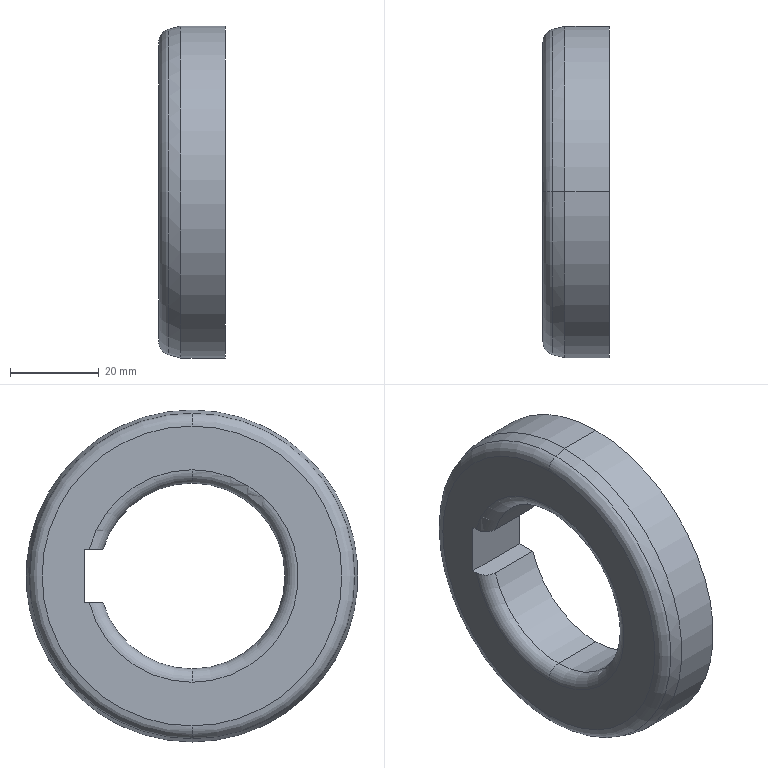Part | STEP file | Input 96 | 1 solid | 17 faces | box 15 x 75 x 75 mm | volume 43593 mm3 | torus 5 | cylinder 5 | plane 5 | cone 2 | commonest cylinder face diameters 42 x3 75 x2
STEP:
#1=CARTESIAN_POINT('',(0.,0.,0.));
#2=DIRECTION('',(0.,0.,1.));
#3=DIRECTION('',(1.,0.,0.));
#4=AXIS2_PLACEMENT_3D('',#1,#2,#3);
#5=CARTESIAN_POINT('',(3698.,665.,23.594));
#6=VERTEX_POINT('',#5);
#7=CARTESIAN_POINT('',(3698.,665.,-24.406));
#8=VERTEX_POINT('',#7);
#9=CARTESIAN_POINT('',(3698.,665.,-0.4063));
#10=DIRECTION('',(1.,0.,0.));
#11=DIRECTION('',(0.,0.,-1.));
#12=AXIS2_PLACEMENT_3D('',#9,#10,#11);
#13=CIRCLE('',#12,24.);
#14=CARTESIAN_POINT('',(3701.,665.,-0.4063));
#15=DIRECTION('',(-1.,0.,0.));
#16=DIRECTION('',(0.,0.,-1.));
#17=AXIS2_PLACEMENT_3D('',#14,#15,#16);
#18=TOROIDAL_SURFACE('',#17,24.,3.);
#19=CARTESIAN_POINT('',(6.283,1.571));
#20=DIRECTION('',(-1.,0.));
#21=VECTOR('',#20,1.);
#22=LINE('',#19,#21);
#23=(GEOMETRIC_REPRESENTATION_CONTEXT(2)PARAMETRIC_REPRESENTATION_CONTEXT()REPRESENTATION_CONTEXT('',''));
#24=DEFINITIONAL_REPRESENTATION('',(#22),#23);
#25=PCURVE('',#18,#24);
#26=CARTESIAN_POINT('',(3698.,665.,-0.4063));
#27=DIRECTION('',(-1.,0.,0.));
#28=DIRECTION('',(0.,0.,-1.));
#29=AXIS2_PLACEMENT_3D('',#26,#27,#28);
#30=PLANE('',#29);
#31=CARTESIAN_POINT('',(24.,0.));
#32=CARTESIAN_POINT('',(24.,-41.569));
#33=CARTESIAN_POINT('',(-12.,-20.785));
#34=CARTESIAN_POINT('',(-48.,0.));
#35=CARTESIAN_POINT('',(-12.,20.785));
#36=CARTESIAN_POINT('',(24.,41.569));
#37=CARTESIAN_POINT('',(24.,0.));
#38=(BOUNDED_CURVE()B_SPLINE_CURVE(2,(#31,#32,#33,#34,#35,#36,#37),.UNSPECIFIED.,.T.,.F.)B_SPLINE_CURVE_WITH_KNOTS((1,2,2,2,2,1),(-2.094,0.,2.094,4.189,6.283,8.378),.UNSPECIFIED.)CURVE()GEOMETRIC_REPRESENTATION_ITEM()RATIONAL_B_SPLINE_CURVE((1.,0.5,1.,0.5,1.,0.5,1.))REPRESENTATION_ITEM(''));
#39=(GEOMETRIC_REPRESENTATION_CONTEXT(2)PARAMETRIC_REPRESENTATION_CONTEXT()REPRESENTATION_CONTEXT('',''));
#40=DEFINITIONAL_REPRESENTATION('',(#38),#39);
#41=PCURVE('',#30,#40);
#42=SURFACE_CURVE('',#13,(#25,#41),.PCURVE_S1.);
#43=EDGE_CURVE('',#6,#8,#42,.T.);
#44=ORIENTED_EDGE('',*,*,#43,.F.);
#45=CARTESIAN_POINT('',(3701.,665.,20.594));
#46=VERTEX_POINT('',#45);
#47=CARTESIAN_POINT('',(3701.,665.,23.594));
#48=DIRECTION('',(0.,-1.,0.));
#49=DIRECTION('',(0.,0.,-1.));
#50=AXIS2_PLACEMENT_3D('',#47,#48,#49);
#51=CIRCLE('',#50,3.);
#52=CARTESIAN_POINT('',(3.142,-3.142));
#53=DIRECTION('',(0.,1.));
#54=VECTOR('',#53,1.);
#55=LINE('',#52,#54);
#56=(GEOMETRIC_REPRESENTATION_CONTEXT(2)PARAMETRIC_REPRESENTATION_CONTEXT()REPRESENTATION_CONTEXT('',''));
#57=DEFINITIONAL_REPRESENTATION('',(#55),#56);
#58=PCURVE('',#18,#57);
#59=CARTESIAN_POINT('',(3701.,665.,-0.4063));
#60=DIRECTION('',(-1.,0.,0.));
#61=DIRECTION('',(0.,0.,-1.));
#62=AXIS2_PLACEMENT_3D('',#59,#60,#61);
#63=TOROIDAL_SURFACE('',#62,24.,3.);
#64=CARTESIAN_POINT('',(3.142,-3.142));
#65=DIRECTION('',(0.,1.));
#66=VECTOR('',#65,1.);
#67=LINE('',#64,#66);
#68=(GEOMETRIC_REPRESENTATION_CONTEXT(2)PARAMETRIC_REPRESENTATION_CONTEXT()REPRESENTATION_CONTEXT('',''));
#69=DEFINITIONAL_REPRESENTATION('',(#67),#68);
#70=PCURVE('',#63,#69);
#71=SURFACE_CURVE('',#51,(#58,#70),.PCURVE_S1.);
#72=EDGE_CURVE('',#6,#46,#71,.T.);
#73=ORIENTED_EDGE('',*,*,#72,.T.);
#74=CARTESIAN_POINT('',(3701.,665.,-21.406));
#75=VERTEX_POINT('',#74);
#76=CARTESIAN_POINT('',(3701.,665.,-0.4063));
#77=DIRECTION('',(-1.,0.,0.));
#78=DIRECTION('',(0.,0.,-1.));
#79=AXIS2_PLACEMENT_3D('',#76,#77,#78);
#80=CIRCLE('',#79,21.);
#81=CARTESIAN_POINT('',(0.,3.142));
#82=DIRECTION('',(1.,0.));
#83=VECTOR('',#82,1.);
#84=LINE('',#81,#83);
#85=(GEOMETRIC_REPRESENTATION_CONTEXT(2)PARAMETRIC_REPRESENTATION_CONTEXT()REPRESENTATION_CONTEXT('',''));
#86=DEFINITIONAL_REPRESENTATION('',(#84),#85);
#87=PCURVE('',#18,#86);
#88=CARTESIAN_POINT('',(3698.,665.,-0.4063));
#89=DIRECTION('',(-1.,0.,0.));
#90=DIRECTION('',(0.,0.,-1.));
#91=AXIS2_PLACEMENT_3D('',#88,#89,#90);
#92=CYLINDRICAL_SURFACE('',#91,21.);
#93=CARTESIAN_POINT('',(0.,-3.));
#94=DIRECTION('',(1.,0.));
#95=VECTOR('',#94,1.);
#96=LINE('',#93,#95);
#97=(GEOMETRIC_REPRESENTATION_CONTEXT(2)PARAMETRIC_REPRESENTATION_CONTEXT()REPRESENTATION_CONTEXT('',''));
#98=DEFINITIONAL_REPRESENTATION('',(#96),#97);
#99=PCURVE('',#92,#98);
#100=SURFACE_CURVE('',#80,(#87,#99),.PCURVE_S1.);
#101=EDGE_CURVE('',#75,#46,#100,.T.);
#102=ORIENTED_EDGE('',*,*,#101,.F.);
#103=CARTESIAN_POINT('',(3701.,665.,-24.406));
#104=DIRECTION('',(0.,1.,0.));
#105=DIRECTION('',(0.,0.,1.));
#106=AXIS2_PLACEMENT_3D('',#103,#104,#105);
#107=CIRCLE('',#106,3.);
#108=CARTESIAN_POINT('',(0.,-3.142));
#109=DIRECTION('',(0.,1.));
#110=VECTOR('',#109,1.);
#111=LINE('',#108,#110);
#112=(GEOMETRIC_REPRESENTATION_CONTEXT(2)PARAMETRIC_REPRESENTATION_CONTEXT()REPRESENTATION_CONTEXT('',''));
#113=DEFINITIONAL_REPRESENTATION('',(#111),#112);
#114=PCURVE('',#18,#113);
#115=CARTESIAN_POINT('',(3701.,665.,-0.4063));
#116=DIRECTION('',(-1.,0.,0.));
#117=DIRECTION('',(0.,0.,-1.));
#118=AXIS2_PLACEMENT_3D('',#115,#116,#117);
#119=TOROIDAL_SURFACE('',#118,24.,3.);
#120=CARTESIAN_POINT('',(6.283,-3.142));
#121=DIRECTION('',(0.,1.));
#122=VECTOR('',#121,1.);
#123=LINE('',#120,#122);
#124=(GEOMETRIC_REPRESENTATION_CONTEXT(2)PARAMETRIC_REPRESENTATION_CONTEXT()REPRESENTATION_CONTEXT('',''));
#125=DEFINITIONAL_REPRESENTATION('',(#123),#124);
#126=PCURVE('',#119,#125);
#127=SURFACE_CURVE('',#107,(#114,#126),.PCURVE_S1.);
#128=EDGE_CURVE('',#8,#75,#127,.T.);
#129=ORIENTED_EDGE('',*,*,#128,.F.);
#130=EDGE_LOOP('',(#44,#73,#102,#129));
#131=FACE_BOUND('',#130,.T.);
#132=ADVANCED_FACE('',(#131),#18,.T.);
#133=CARTESIAN_POINT('',(3698.,688.238,-6.406));
#134=VERTEX_POINT('',#133);
#135=CARTESIAN_POINT('',(3698.,665.,-0.4063));
#136=DIRECTION('',(1.,0.,0.));
#137=DIRECTION('',(0.,0.,-1.));
#138=AXIS2_PLACEMENT_3D('',#135,#136,#137);
#139=CIRCLE('',#138,24.);
#140=CARTESIAN_POINT('',(6.283,1.571));
#141=DIRECTION('',(-1.,0.));
#142=VECTOR('',#141,1.);
#143=LINE('',#140,#142);
#144=(GEOMETRIC_REPRESENTATION_CONTEXT(2)PARAMETRIC_REPRESENTATION_CONTEXT()REPRESENTATION_CONTEXT('',''));
#145=DEFINITIONAL_REPRESENTATION('',(#143),#144);
#146=PCURVE('',#119,#145);
#147=CARTESIAN_POINT('',(24.,0.));
#148=CARTESIAN_POINT('',(24.,-41.569));
#149=CARTESIAN_POINT('',(-12.,-20.785));
#150=CARTESIAN_POINT('',(-48.,0.));
#151=CARTESIAN_POINT('',(-12.,20.785));
#152=CARTESIAN_POINT('',(24.,41.569));
#153=CARTESIAN_POINT('',(24.,0.));
#154=(BOUNDED_CURVE()B_SPLINE_CURVE(2,(#147,#148,#149,#150,#151,#152,#153),.UNSPECIFIED.,.T.,.F.)B_SPLINE_CURVE_WITH_KNOTS((1,2,2,2,2,1),(-2.094,0.,2.094,4.189,6.283,8.378),.UNSPECIFIED.)CURVE()GEOMETRIC_REPRESENTATION_ITEM()RATIONAL_B_SPLINE_CURVE((1.,0.5,1.,0.5,1.,0.5,1.))REPRESENTATION_ITEM(''));
#155=(GEOMETRIC_REPRESENTATION_CONTEXT(2)PARAMETRIC_REPRESENTATION_CONTEXT()REPRESENTATION_CONTEXT('',''));
#156=DEFINITIONAL_REPRESENTATION('',(#154),#155);
#157=PCURVE('',#30,#156);
#158=SURFACE_CURVE('',#139,(#146,#157),.PCURVE_S1.);
#159=EDGE_CURVE('',#8,#134,#158,.T.);
#160=ORIENTED_EDGE('',*,*,#159,.F.);
#161=ORIENTED_EDGE('',*,*,#128,.T.);
#162=CARTESIAN_POINT('',(3701.,685.125,-6.406));
#163=VERTEX_POINT('',#162);
#164=CARTESIAN_POINT('',(3701.,665.,-0.4063));
#165=DIRECTION('',(-1.,0.,0.));
#166=DIRECTION('',(0.,0.,-1.));
#167=AXIS2_PLACEMENT_3D('',#164,#165,#166);
#168=CIRCLE('',#167,21.);
#169=CARTESIAN_POINT('',(0.,3.142));
#170=DIRECTION('',(1.,0.));
#171=VECTOR('',#170,1.);
#172=LINE('',#169,#171);
#173=(GEOMETRIC_REPRESENTATION_CONTEXT(2)PARAMETRIC_REPRESENTATION_CONTEXT()REPRESENTATION_CONTEXT('',''));
#174=DEFINITIONAL_REPRESENTATION('',(#172),#173);
#175=PCURVE('',#119,#174);
#176=CARTESIAN_POINT('',(3698.,665.,-0.4063));
#177=DIRECTION('',(-1.,0.,0.));
#178=DIRECTION('',(0.,0.,-1.));
#179=AXIS2_PLACEMENT_3D('',#176,#177,#178);
#180=CYLINDRICAL_SURFACE('',#179,21.);
#181=CARTESIAN_POINT('',(0.,-3.));
#182=DIRECTION('',(1.,0.));
#183=VECTOR('',#182,1.);
#184=LINE('',#181,#183);
#185=(GEOMETRIC_REPRESENTATION_CONTEXT(2)PARAMETRIC_REPRESENTATION_CONTEXT()REPRESENTATION_CONTEXT('',''));
#186=DEFINITIONAL_REPRESENTATION('',(#184),#185);
#187=PCURVE('',#180,#186);
#188=SURFACE_CURVE('',#168,(#175,#187),.PCURVE_S1.);
#189=EDGE_CURVE('',#163,#75,#188,.T.);
#190=ORIENTED_EDGE('',*,*,#189,.F.);
#191=CARTESIAN_POINT('',(3698.,688.238,-6.406));
#192=CARTESIAN_POINT('',(3698.,688.036,-6.406));
#193=CARTESIAN_POINT('',(3698.019,687.838,-6.406));
#194=CARTESIAN_POINT('',(3698.093,687.447,-6.406));
#195=CARTESIAN_POINT('',(3698.149,687.253,-6.406));
#196=CARTESIAN_POINT('',(3698.296,686.879,-6.406));
#197=CARTESIAN_POINT('',(3698.386,686.702,-6.406));
#198=CARTESIAN_POINT('',(3698.598,686.365,-6.406));
#199=CARTESIAN_POINT('',(3698.723,686.204,-6.406));
#200=CARTESIAN_POINT('',(3698.997,685.914,-6.406));
#201=CARTESIAN_POINT('',(3699.147,685.784,-6.406));
#202=CARTESIAN_POINT('',(3699.473,685.552,-6.406));
#203=CARTESIAN_POINT('',(3699.65,685.452,-6.406));
#204=CARTESIAN_POINT('',(3700.196,685.211,-6.406));
#205=CARTESIAN_POINT('',(3700.596,685.125,-6.406));
#206=CARTESIAN_POINT('',(3701.,685.125,-6.406));
#207=B_SPLINE_CURVE_WITH_KNOTS('',3,(#191,#192,#193,#194,#195,#196,#197,#198,#199,#200,#201,#202,#203,#204,#205,#206),.UNSPECIFIED.,.F.,.F.,(4,2,2,2,2,2,2,4),(0.,0.0005967,0.001193,0.00179,0.002387,0.002984,0.00358,0.004774),.UNSPECIFIED.);
#208=CARTESIAN_POINT('',(4.965,1.571));
#209=CARTESIAN_POINT('',(4.965,1.583));
#210=CARTESIAN_POINT('',(4.966,1.606));
#211=CARTESIAN_POINT('',(4.967,1.641));
#212=CARTESIAN_POINT('',(4.969,1.677));
#213=CARTESIAN_POINT('',(4.97,1.712));
#214=CARTESIAN_POINT('',(4.971,1.747));
#215=CARTESIAN_POINT('',(4.972,1.782));
#216=CARTESIAN_POINT('',(4.973,1.817));
#217=CARTESIAN_POINT('',(4.974,1.852));
#218=CARTESIAN_POINT('',(4.976,1.887));
#219=CARTESIAN_POINT('',(4.977,1.923));
#220=CARTESIAN_POINT('',(4.978,1.958));
#221=CARTESIAN_POINT('',(4.979,1.993));
#222=CARTESIAN_POINT('',(4.98,2.029));
#223=CARTESIAN_POINT('',(4.981,2.064));
#224=CARTESIAN_POINT('',(4.982,2.099));
#225=CARTESIAN_POINT('',(4.984,2.134));
#226=CARTESIAN_POINT('',(4.985,2.169));
#227=CARTESIAN_POINT('',(4.986,2.205));
#228=CARTESIAN_POINT('',(4.987,2.24));
#229=CARTESIAN_POINT('',(4.988,2.276));
#230=CARTESIAN_POINT('',(4.989,2.312));
#231=CARTESIAN_POINT('',(4.99,2.347));
#232=CARTESIAN_POINT('',(4.991,2.383));
#233=CARTESIAN_POINT('',(4.992,2.418));
#234=CARTESIAN_POINT('',(4.993,2.454));
#235=CARTESIAN_POINT('',(4.994,2.49));
#236=CARTESIAN_POINT('',(4.995,2.525));
#237=CARTESIAN_POINT('',(4.995,2.561));
#238=CARTESIAN_POINT('',(4.996,2.597));
#239=CARTESIAN_POINT('',(4.997,2.633));
#240=CARTESIAN_POINT('',(4.998,2.669));
#241=CARTESIAN_POINT('',(4.998,2.706));
#242=CARTESIAN_POINT('',(4.999,2.742));
#243=CARTESIAN_POINT('',(4.999,2.778));
#244=CARTESIAN_POINT('',(5.,2.814));
#245=CARTESIAN_POINT('',(5.,2.85));
#246=CARTESIAN_POINT('',(5.001,2.886));
#247=CARTESIAN_POINT('',(5.001,2.922));
#248=CARTESIAN_POINT('',(5.001,2.959));
#249=CARTESIAN_POINT('',(5.002,2.995));
#250=CARTESIAN_POINT('',(5.002,3.032));
#251=CARTESIAN_POINT('',(5.002,3.068));
#252=CARTESIAN_POINT('',(5.002,3.105));
#253=CARTESIAN_POINT('',(5.002,3.129));
#254=CARTESIAN_POINT('',(5.002,3.142));
#255=B_SPLINE_CURVE_WITH_KNOTS('',3,(#208,#209,#210,#211,#212,#213,#214,#215,#216,#217,#218,#219,#220,#221,#222,#223,#224,#225,#226,#227,#228,#229,#230,#231,#232,#233,#234,#235,#236,#237,#238,#239,#240,#241,#242,#243,#244,#245,#246,#247,#248,#249,#250,#251,#252,#253,#254),.UNSPECIFIED.,.F.,.F.,(4,1,1,1,1,1,1,1,1,1,1,1,1,1,1,1,1,1,1,1,1,1,1,1,1,1,1,1,1,1,1,1,1,1,1,1,1,1,1,1,1,1,1,1,4),(0.,0.0001085,0.000217,0.0003255,0.000434,0.0005425,0.0006509,0.0007594,0.0008679,0.0009764,0.001085,0.001193,0.001302,0.00141,0.001519,0.001627,0.001736,0.001844,0.001953,0.002061,0.00217,0.002278,0.002387,0.002495,0.002604,0.002712,0.002821,0.002929,0.003038,0.003146,0.003255,0.003363,0.003472,0.00358,0.003689,0.003797,0.003906,0.004014,0.004123,0.004231,0.00434,0.004448,0.004557,0.004665,0.004774),.QUASI_UNIFORM_KNOTS.);
#256=(GEOMETRIC_REPRESENTATION_CONTEXT(2)PARAMETRIC_REPRESENTATION_CONTEXT()REPRESENTATION_CONTEXT('',''));
#257=DEFINITIONAL_REPRESENTATION('',(#255),#256);
#258=PCURVE('',#119,#257);
#259=CARTESIAN_POINT('',(3803.,665.,-6.406));
#260=DIRECTION('',(0.,0.,1.));
#261=DIRECTION('',(0.,-1.,0.));
#262=AXIS2_PLACEMENT_3D('',#259,#260,#261);
#263=PLANE('',#262);
#264=CARTESIAN_POINT('',(-23.238,-105.));
#265=CARTESIAN_POINT('',(-23.036,-105.));
#266=CARTESIAN_POINT('',(-22.838,-104.981));
#267=CARTESIAN_POINT('',(-22.447,-104.907));
#268=CARTESIAN_POINT('',(-22.253,-104.851));
#269=CARTESIAN_POINT('',(-21.879,-104.704));
#270=CARTESIAN_POINT('',(-21.702,-104.614));
#271=CARTESIAN_POINT('',(-21.365,-104.402));
#272=CARTESIAN_POINT('',(-21.204,-104.277));
#273=CARTESIAN_POINT('',(-20.914,-104.003));
#274=CARTESIAN_POINT('',(-20.784,-103.853));
#275=CARTESIAN_POINT('',(-20.552,-103.527));
#276=CARTESIAN_POINT('',(-20.452,-103.35));
#277=CARTESIAN_POINT('',(-20.211,-102.804));
#278=CARTESIAN_POINT('',(-20.125,-102.404));
#279=CARTESIAN_POINT('',(-20.125,-102.));
#280=B_SPLINE_CURVE_WITH_KNOTS('',3,(#264,#265,#266,#267,#268,#269,#270,#271,#272,#273,#274,#275,#276,#277,#278,#279),.UNSPECIFIED.,.F.,.F.,(4,2,2,2,2,2,2,4),(0.,0.0005967,0.001193,0.00179,0.002387,0.002984,0.00358,0.004774),.UNSPECIFIED.);
#281=(GEOMETRIC_REPRESENTATION_CONTEXT(2)PARAMETRIC_REPRESENTATION_CONTEXT()REPRESENTATION_CONTEXT('',''));
#282=DEFINITIONAL_REPRESENTATION('',(#280),#281);
#283=PCURVE('',#263,#282);
#284=SURFACE_CURVE('',#207,(#258,#283),.PCURVE_S1.);
#285=EDGE_CURVE('',#134,#163,#284,.T.);
#286=ORIENTED_EDGE('',*,*,#285,.F.);
#287=EDGE_LOOP('',(#160,#161,#190,#286));
#288=FACE_BOUND('',#287,.T.);
#289=ADVANCED_FACE('',(#288),#119,.T.);
#290=CARTESIAN_POINT('',(3700.224,665.,36.35));
#291=VERTEX_POINT('',#290);
#292=CARTESIAN_POINT('',(3700.224,665.,-37.162));
#293=VERTEX_POINT('',#292);
#294=CARTESIAN_POINT('',(3700.224,665.,-0.4063));
#295=DIRECTION('',(1.,0.,0.));
#296=DIRECTION('',(0.,0.,-1.));
#297=AXIS2_PLACEMENT_3D('',#294,#295,#296);
#298=CIRCLE('',#297,36.756);
#299=CARTESIAN_POINT('',(3701.,665.,-0.4063));
#300=DIRECTION('',(-1.,0.,0.));
#301=DIRECTION('',(0.,0.,-1.));
#302=AXIS2_PLACEMENT_3D('',#299,#300,#301);
#303=TOROIDAL_SURFACE('',#302,33.858,3.);
#304=CARTESIAN_POINT('',(6.283,0.2618));
#305=DIRECTION('',(-1.,0.));
#306=VECTOR('',#305,1.);
#307=LINE('',#304,#306);
#308=(GEOMETRIC_REPRESENTATION_CONTEXT(2)PARAMETRIC_REPRESENTATION_CONTEXT()REPRESENTATION_CONTEXT('',''));
#309=DEFINITIONAL_REPRESENTATION('',(#307),#308);
#310=PCURVE('',#303,#309);
#311=CARTESIAN_POINT('',(3703.,665.,-0.4063));
#312=DIRECTION('',(1.,0.,0.));
#313=DIRECTION('',(0.,0.,1.));
#314=AXIS2_PLACEMENT_3D('',#311,#312,#313);
#315=CONICAL_SURFACE('',#314,37.5,0.2618);
#316=CARTESIAN_POINT('',(-3.142,-2.776));
#317=DIRECTION('',(1.,0.));
#318=VECTOR('',#317,1.);
#319=LINE('',#316,#318);
#320=(GEOMETRIC_REPRESENTATION_CONTEXT(2)PARAMETRIC_REPRESENTATION_CONTEXT()REPRESENTATION_CONTEXT('',''));
#321=DEFINITIONAL_REPRESENTATION('',(#319),#320);
#322=PCURVE('',#315,#321);
#323=SURFACE_CURVE('',#298,(#310,#322),.PCURVE_S1.);
#324=EDGE_CURVE('',#291,#293,#323,.T.);
#325=ORIENTED_EDGE('',*,*,#324,.F.);
#326=CARTESIAN_POINT('',(3698.,665.,33.452));
#327=VERTEX_POINT('',#326);
#328=CARTESIAN_POINT('',(3701.,665.,33.452));
#329=DIRECTION('',(0.,-1.,0.));
#330=DIRECTION('',(0.,0.,-1.));
#331=AXIS2_PLACEMENT_3D('',#328,#329,#330);
#332=CIRCLE('',#331,3.);
#333=CARTESIAN_POINT('',(3.142,-3.142));
#334=DIRECTION('',(0.,1.));
#335=VECTOR('',#334,1.);
#336=LINE('',#333,#335);
#337=(GEOMETRIC_REPRESENTATION_CONTEXT(2)PARAMETRIC_REPRESENTATION_CONTEXT()REPRESENTATION_CONTEXT('',''));
#338=DEFINITIONAL_REPRESENTATION('',(#336),#337);
#339=PCURVE('',#303,#338);
#340=CARTESIAN_POINT('',(3701.,665.,-0.4063));
#341=DIRECTION('',(-1.,0.,0.));
#342=DIRECTION('',(0.,0.,-1.));
#343=AXIS2_PLACEMENT_3D('',#340,#341,#342);
#344=TOROIDAL_SURFACE('',#343,33.858,3.);
#345=CARTESIAN_POINT('',(3.142,-3.142));
#346=DIRECTION('',(0.,1.));
#347=VECTOR('',#346,1.);
#348=LINE('',#345,#347);
#349=(GEOMETRIC_REPRESENTATION_CONTEXT(2)PARAMETRIC_REPRESENTATION_CONTEXT()REPRESENTATION_CONTEXT('',''));
#350=DEFINITIONAL_REPRESENTATION('',(#348),#349);
#351=PCURVE('',#344,#350);
#352=SURFACE_CURVE('',#332,(#339,#351),.PCURVE_S1.);
#353=EDGE_CURVE('',#291,#327,#352,.T.);
#354=ORIENTED_EDGE('',*,*,#353,.T.);
#355=CARTESIAN_POINT('',(3698.,665.,-34.265));
#356=VERTEX_POINT('',#355);
#357=CARTESIAN_POINT('',(3698.,665.,-0.4063));
#358=DIRECTION('',(-1.,0.,0.));
#359=DIRECTION('',(0.,0.,-1.));
#360=AXIS2_PLACEMENT_3D('',#357,#358,#359);
#361=CIRCLE('',#360,33.858);
#362=CARTESIAN_POINT('',(0.,1.571));
#363=DIRECTION('',(1.,0.));
#364=VECTOR('',#363,1.);
#365=LINE('',#362,#364);
#366=(GEOMETRIC_REPRESENTATION_CONTEXT(2)PARAMETRIC_REPRESENTATION_CONTEXT()REPRESENTATION_CONTEXT('',''));
#367=DEFINITIONAL_REPRESENTATION('',(#365),#366);
#368=PCURVE('',#303,#367);
#369=CARTESIAN_POINT('',(0.,0.));
#370=DIRECTION('',(1.,0.));
#371=AXIS2_PLACEMENT_2D('',#369,#370);
#372=CIRCLE('',#371,33.858);
#373=(GEOMETRIC_REPRESENTATION_CONTEXT(2)PARAMETRIC_REPRESENTATION_CONTEXT()REPRESENTATION_CONTEXT('',''));
#374=DEFINITIONAL_REPRESENTATION('',(#372),#373);
#375=PCURVE('',#30,#374);
#376=SURFACE_CURVE('',#361,(#368,#375),.PCURVE_S1.);
#377=EDGE_CURVE('',#356,#327,#376,.T.);
#378=ORIENTED_EDGE('',*,*,#377,.F.);
#379=CARTESIAN_POINT('',(3701.,665.,-34.265));
#380=DIRECTION('',(0.,1.,0.));
#381=DIRECTION('',(0.,0.,1.));
#382=AXIS2_PLACEMENT_3D('',#379,#380,#381);
#383=CIRCLE('',#382,3.);
#384=CARTESIAN_POINT('',(0.,-3.142));
#385=DIRECTION('',(0.,1.));
#386=VECTOR('',#385,1.);
#387=LINE('',#384,#386);
#388=(GEOMETRIC_REPRESENTATION_CONTEXT(2)PARAMETRIC_REPRESENTATION_CONTEXT()REPRESENTATION_CONTEXT('',''));
#389=DEFINITIONAL_REPRESENTATION('',(#387),#388);
#390=PCURVE('',#303,#389);
#391=CARTESIAN_POINT('',(6.283,-3.142));
#392=DIRECTION('',(0.,1.));
#393=VECTOR('',#392,1.);
#394=LINE('',#391,#393);
#395=(GEOMETRIC_REPRESENTATION_CONTEXT(2)PARAMETRIC_REPRESENTATION_CONTEXT()REPRESENTATION_CONTEXT('',''));
#396=DEFINITIONAL_REPRESENTATION('',(#394),#395);
#397=PCURVE('',#344,#396);
#398=SURFACE_CURVE('',#383,(#390,#397),.PCURVE_S1.);
#399=EDGE_CURVE('',#293,#356,#398,.T.);
#400=ORIENTED_EDGE('',*,*,#399,.F.);
#401=EDGE_LOOP('',(#325,#354,#378,#400));
#402=FACE_BOUND('',#401,.T.);
#403=ADVANCED_FACE('',(#402),#303,.T.);
#404=ORIENTED_EDGE('',*,*,#324,.T.);
#405=CARTESIAN_POINT('',(3703.,665.,-37.906));
#406=VERTEX_POINT('',#405);
#407=CARTESIAN_POINT('',(3703.,665.,-37.906));
#408=DIRECTION('',(0.9659,0.,-0.2588));
#409=VECTOR('',#408,1.);
#410=LINE('',#407,#409);
#411=CARTESIAN_POINT('',(3.142,0.));
#412=DIRECTION('',(0.,1.));
#413=VECTOR('',#412,1.);
#414=LINE('',#411,#413);
#415=(GEOMETRIC_REPRESENTATION_CONTEXT(2)PARAMETRIC_REPRESENTATION_CONTEXT()REPRESENTATION_CONTEXT('',''));
#416=DEFINITIONAL_REPRESENTATION('',(#414),#415);
#417=PCURVE('',#315,#416);
#418=CARTESIAN_POINT('',(3703.,665.,-0.4063));
#419=DIRECTION('',(1.,0.,0.));
#420=DIRECTION('',(0.,0.,1.));
#421=AXIS2_PLACEMENT_3D('',#418,#419,#420);
#422=CONICAL_SURFACE('',#421,37.5,0.2618);
#423=CARTESIAN_POINT('',(3.142,0.));
#424=DIRECTION('',(0.,1.));
#425=VECTOR('',#424,1.);
#426=LINE('',#423,#425);
#427=(GEOMETRIC_REPRESENTATION_CONTEXT(2)PARAMETRIC_REPRESENTATION_CONTEXT()REPRESENTATION_CONTEXT('',''));
#428=DEFINITIONAL_REPRESENTATION('',(#426),#427);
#429=PCURVE('',#422,#428);
#430=SURFACE_CURVE('',#410,(#417,#429),.PCURVE_S1.);
#431=EDGE_CURVE('',#293,#406,#430,.T.);
#432=ORIENTED_EDGE('',*,*,#431,.T.);
#433=CARTESIAN_POINT('',(3703.,665.,37.094));
#434=VERTEX_POINT('',#433);
#435=CARTESIAN_POINT('',(3703.,665.,-0.4063));
#436=DIRECTION('',(1.,0.,0.));
#437=DIRECTION('',(0.,0.,-1.));
#438=AXIS2_PLACEMENT_3D('',#435,#436,#437);
#439=CIRCLE('',#438,37.5);
#440=CARTESIAN_POINT('',(-3.142,0.));
#441=DIRECTION('',(1.,0.));
#442=VECTOR('',#441,1.);
#443=LINE('',#440,#442);
#444=(GEOMETRIC_REPRESENTATION_CONTEXT(2)PARAMETRIC_REPRESENTATION_CONTEXT()REPRESENTATION_CONTEXT('',''));
#445=DEFINITIONAL_REPRESENTATION('',(#443),#444);
#446=PCURVE('',#315,#445);
#447=CARTESIAN_POINT('',(3698.,665.,-0.4063));
#448=DIRECTION('',(1.,0.,0.));
#449=DIRECTION('',(0.,0.,1.));
#450=AXIS2_PLACEMENT_3D('',#447,#448,#449);
#451=CYLINDRICAL_SURFACE('',#450,37.5);
#452=CARTESIAN_POINT('',(-3.142,5.));
#453=DIRECTION('',(1.,0.));
#454=VECTOR('',#453,1.);
#455=LINE('',#452,#454);
#456=(GEOMETRIC_REPRESENTATION_CONTEXT(2)PARAMETRIC_REPRESENTATION_CONTEXT()REPRESENTATION_CONTEXT('',''));
#457=DEFINITIONAL_REPRESENTATION('',(#455),#456);
#458=PCURVE('',#451,#457);
#459=SURFACE_CURVE('',#439,(#446,#458),.PCURVE_S1.);
#460=EDGE_CURVE('',#434,#406,#459,.T.);
#461=ORIENTED_EDGE('',*,*,#460,.F.);
#462=CARTESIAN_POINT('',(3703.,665.,37.094));
#463=DIRECTION('',(0.9659,0.,0.2588));
#464=VECTOR('',#463,1.);
#465=LINE('',#462,#464);
#466=CARTESIAN_POINT('',(0.,0.));
#467=DIRECTION('',(0.,1.));
#468=VECTOR('',#467,1.);
#469=LINE('',#466,#468);
#470=(GEOMETRIC_REPRESENTATION_CONTEXT(2)PARAMETRIC_REPRESENTATION_CONTEXT()REPRESENTATION_CONTEXT('',''));
#471=DEFINITIONAL_REPRESENTATION('',(#469),#470);
#472=PCURVE('',#315,#471);
#473=CARTESIAN_POINT('',(6.283,0.));
#474=DIRECTION('',(0.,1.));
#475=VECTOR('',#474,1.);
#476=LINE('',#473,#475);
#477=(GEOMETRIC_REPRESENTATION_CONTEXT(2)PARAMETRIC_REPRESENTATION_CONTEXT()REPRESENTATION_CONTEXT('',''));
#478=DEFINITIONAL_REPRESENTATION('',(#476),#477);
#479=PCURVE('',#422,#478);
#480=SURFACE_CURVE('',#465,(#472,#479),.PCURVE_S1.);
#481=EDGE_CURVE('',#291,#434,#480,.T.);
#482=ORIENTED_EDGE('',*,*,#481,.F.);
#483=EDGE_LOOP('',(#404,#432,#461,#482));
#484=FACE_BOUND('',#483,.T.);
#485=ADVANCED_FACE('',(#484),#315,.T.);
#486=ORIENTED_EDGE('',*,*,#460,.T.);
#487=CARTESIAN_POINT('',(3713.,665.,-37.906));
#488=VERTEX_POINT('',#487);
#489=CARTESIAN_POINT('',(3698.,665.,-37.906));
#490=DIRECTION('',(1.,0.,0.));
#491=VECTOR('',#490,1.);
#492=LINE('',#489,#491);
#493=CARTESIAN_POINT('',(3.142,0.));
#494=DIRECTION('',(0.,1.));
#495=VECTOR('',#494,1.);
#496=LINE('',#493,#495);
#497=(GEOMETRIC_REPRESENTATION_CONTEXT(2)PARAMETRIC_REPRESENTATION_CONTEXT()REPRESENTATION_CONTEXT('',''));
#498=DEFINITIONAL_REPRESENTATION('',(#496),#497);
#499=PCURVE('',#451,#498);
#500=CARTESIAN_POINT('',(3698.,665.,-0.4063));
#501=DIRECTION('',(1.,0.,0.));
#502=DIRECTION('',(0.,0.,1.));
#503=AXIS2_PLACEMENT_3D('',#500,#501,#502);
#504=CYLINDRICAL_SURFACE('',#503,37.5);
#505=CARTESIAN_POINT('',(3.142,0.));
#506=DIRECTION('',(0.,1.));
#507=VECTOR('',#506,1.);
#508=LINE('',#505,#507);
#509=(GEOMETRIC_REPRESENTATION_CONTEXT(2)PARAMETRIC_REPRESENTATION_CONTEXT()REPRESENTATION_CONTEXT('',''));
#510=DEFINITIONAL_REPRESENTATION('',(#508),#509);
#511=PCURVE('',#504,#510);
#512=SURFACE_CURVE('',#492,(#499,#511),.PCURVE_S1.);
#513=EDGE_CURVE('',#406,#488,#512,.T.);
#514=ORIENTED_EDGE('',*,*,#513,.T.);
#515=CARTESIAN_POINT('',(3713.,665.,37.094));
#516=VERTEX_POINT('',#515);
#517=CARTESIAN_POINT('',(3713.,665.,-0.4063));
#518=DIRECTION('',(1.,0.,0.));
#519=DIRECTION('',(0.,0.,-1.));
#520=AXIS2_PLACEMENT_3D('',#517,#518,#519);
#521=CIRCLE('',#520,37.5);
#522=CARTESIAN_POINT('',(-3.142,15.));
#523=DIRECTION('',(1.,0.));
#524=VECTOR('',#523,1.);
#525=LINE('',#522,#524);
#526=(GEOMETRIC_REPRESENTATION_CONTEXT(2)PARAMETRIC_REPRESENTATION_CONTEXT()REPRESENTATION_CONTEXT('',''));
#527=DEFINITIONAL_REPRESENTATION('',(#525),#526);
#528=PCURVE('',#451,#527);
#529=CARTESIAN_POINT('',(3713.,665.,-0.4063));
#530=DIRECTION('',(-1.,0.,0.));
#531=DIRECTION('',(0.,0.,-1.));
#532=AXIS2_PLACEMENT_3D('',#529,#530,#531);
#533=PLANE('',#532);
#534=CARTESIAN_POINT('',(37.5,0.));
#535=CARTESIAN_POINT('',(37.5,-64.952));
#536=CARTESIAN_POINT('',(-18.75,-32.476));
#537=CARTESIAN_POINT('',(-75.,0.));
#538=CARTESIAN_POINT('',(-18.75,32.476));
#539=CARTESIAN_POINT('',(37.5,64.952));
#540=CARTESIAN_POINT('',(37.5,0.));
#541=(BOUNDED_CURVE()B_SPLINE_CURVE(2,(#534,#535,#536,#537,#538,#539,#540),.UNSPECIFIED.,.T.,.F.)B_SPLINE_CURVE_WITH_KNOTS((1,2,2,2,2,1),(-2.094,0.,2.094,4.189,6.283,8.378),.UNSPECIFIED.)CURVE()GEOMETRIC_REPRESENTATION_ITEM()RATIONAL_B_SPLINE_CURVE((1.,0.5,1.,0.5,1.,0.5,1.))REPRESENTATION_ITEM(''));
#542=(GEOMETRIC_REPRESENTATION_CONTEXT(2)PARAMETRIC_REPRESENTATION_CONTEXT()REPRESENTATION_CONTEXT('',''));
#543=DEFINITIONAL_REPRESENTATION('',(#541),#542);
#544=PCURVE('',#533,#543);
#545=SURFACE_CURVE('',#521,(#528,#544),.PCURVE_S1.);
#546=EDGE_CURVE('',#516,#488,#545,.T.);
#547=ORIENTED_EDGE('',*,*,#546,.F.);
#548=CARTESIAN_POINT('',(3698.,665.,37.094));
#549=DIRECTION('',(1.,0.,0.));
#550=VECTOR('',#549,1.);
#551=LINE('',#548,#550);
#552=CARTESIAN_POINT('',(0.,0.));
#553=DIRECTION('',(0.,1.));
#554=VECTOR('',#553,1.);
#555=LINE('',#552,#554);
#556=(GEOMETRIC_REPRESENTATION_CONTEXT(2)PARAMETRIC_REPRESENTATION_CONTEXT()REPRESENTATION_CONTEXT('',''));
#557=DEFINITIONAL_REPRESENTATION('',(#555),#556);
#558=PCURVE('',#451,#557);
#559=CARTESIAN_POINT('',(6.283,0.));
#560=DIRECTION('',(0.,1.));
#561=VECTOR('',#560,1.);
#562=LINE('',#559,#561);
#563=(GEOMETRIC_REPRESENTATION_CONTEXT(2)PARAMETRIC_REPRESENTATION_CONTEXT()REPRESENTATION_CONTEXT('',''));
#564=DEFINITIONAL_REPRESENTATION('',(#562),#563);
#565=PCURVE('',#504,#564);
#566=SURFACE_CURVE('',#551,(#558,#565),.PCURVE_S1.);
#567=EDGE_CURVE('',#434,#516,#566,.T.);
#568=ORIENTED_EDGE('',*,*,#567,.F.);
#569=EDGE_LOOP('',(#486,#514,#547,#568));
#570=FACE_BOUND('',#569,.T.);
#571=ADVANCED_FACE('',(#570),#451,.T.);
#572=CARTESIAN_POINT('',(3701.,685.125,5.594));
#573=VERTEX_POINT('',#572);
#574=CARTESIAN_POINT('',(3713.,685.125,5.594));
#575=VERTEX_POINT('',#574);
#576=CARTESIAN_POINT('',(3698.,685.125,5.594));
#577=DIRECTION('',(1.,0.,0.));
#578=VECTOR('',#577,1.);
#579=LINE('',#576,#578);
#580=CARTESIAN_POINT('',(3698.,665.,-0.4063));
#581=DIRECTION('',(-1.,0.,0.));
#582=DIRECTION('',(0.,0.,-1.));
#583=AXIS2_PLACEMENT_3D('',#580,#581,#582);
#584=CYLINDRICAL_SURFACE('',#583,21.);
#585=CARTESIAN_POINT('',(4.423,0.));
#586=DIRECTION('',(0.,-1.));
#587=VECTOR('',#586,1.);
#588=LINE('',#585,#587);
#589=(GEOMETRIC_REPRESENTATION_CONTEXT(2)PARAMETRIC_REPRESENTATION_CONTEXT()REPRESENTATION_CONTEXT('',''));
#590=DEFINITIONAL_REPRESENTATION('',(#588),#589);
#591=PCURVE('',#584,#590);
#592=CARTESIAN_POINT('',(3803.,689.3,5.594));
#593=DIRECTION('',(0.,0.,-1.));
#594=DIRECTION('',(1.,0.,0.));
#595=AXIS2_PLACEMENT_3D('',#592,#593,#594);
#596=PLANE('',#595);
#597=CARTESIAN_POINT('',(-105.,4.175));
#598=DIRECTION('',(1.,0.));
#599=VECTOR('',#598,1.);
#600=LINE('',#597,#599);
#601=(GEOMETRIC_REPRESENTATION_CONTEXT(2)PARAMETRIC_REPRESENTATION_CONTEXT()REPRESENTATION_CONTEXT('',''));
#602=DEFINITIONAL_REPRESENTATION('',(#600),#601);
#603=PCURVE('',#596,#602);
#604=SURFACE_CURVE('',#579,(#591,#603),.PCURVE_S1.);
#605=EDGE_CURVE('',#573,#575,#604,.T.);
#606=ORIENTED_EDGE('',*,*,#605,.F.);
#607=CARTESIAN_POINT('',(3701.,665.,-0.4063));
#608=DIRECTION('',(-1.,0.,0.));
#609=DIRECTION('',(0.,0.,-1.));
#610=AXIS2_PLACEMENT_3D('',#607,#608,#609);
#611=CIRCLE('',#610,21.);
#612=CARTESIAN_POINT('',(0.,-3.));
#613=DIRECTION('',(1.,0.));
#614=VECTOR('',#613,1.);
#615=LINE('',#612,#614);
#616=(GEOMETRIC_REPRESENTATION_CONTEXT(2)PARAMETRIC_REPRESENTATION_CONTEXT()REPRESENTATION_CONTEXT('',''));
#617=DEFINITIONAL_REPRESENTATION('',(#615),#616);
#618=PCURVE('',#584,#617);
#619=CARTESIAN_POINT('',(0.,3.142));
#620=DIRECTION('',(1.,0.));
#621=VECTOR('',#620,1.);
#622=LINE('',#619,#621);
#623=(GEOMETRIC_REPRESENTATION_CONTEXT(2)PARAMETRIC_REPRESENTATION_CONTEXT()REPRESENTATION_CONTEXT('',''));
#624=DEFINITIONAL_REPRESENTATION('',(#622),#623);
#625=PCURVE('',#63,#624);
#626=SURFACE_CURVE('',#611,(#618,#625),.PCURVE_S1.);
#627=EDGE_CURVE('',#46,#573,#626,.T.);
#628=ORIENTED_EDGE('',*,*,#627,.F.);
#629=CARTESIAN_POINT('',(3713.,665.,20.594));
#630=VERTEX_POINT('',#629);
#631=CARTESIAN_POINT('',(3698.,665.,20.594));
#632=DIRECTION('',(-1.,0.,0.));
#633=VECTOR('',#632,1.);
#634=LINE('',#631,#633);
#635=CARTESIAN_POINT('',(3.142,0.));
#636=DIRECTION('',(0.,1.));
#637=VECTOR('',#636,1.);
#638=LINE('',#635,#637);
#639=(GEOMETRIC_REPRESENTATION_CONTEXT(2)PARAMETRIC_REPRESENTATION_CONTEXT()REPRESENTATION_CONTEXT('',''));
#640=DEFINITIONAL_REPRESENTATION('',(#638),#639);
#641=PCURVE('',#584,#640);
#642=CARTESIAN_POINT('',(3.142,0.));
#643=DIRECTION('',(0.,1.));
#644=VECTOR('',#643,1.);
#645=LINE('',#642,#644);
#646=(GEOMETRIC_REPRESENTATION_CONTEXT(2)PARAMETRIC_REPRESENTATION_CONTEXT()REPRESENTATION_CONTEXT('',''));
#647=DEFINITIONAL_REPRESENTATION('',(#645),#646);
#648=PCURVE('',#92,#647);
#649=SURFACE_CURVE('',#634,(#641,#648),.PCURVE_S1.);
#650=EDGE_CURVE('',#630,#46,#649,.T.);
#651=ORIENTED_EDGE('',*,*,#650,.F.);
#652=CARTESIAN_POINT('',(3713.,665.,-0.4063));
#653=DIRECTION('',(-1.,0.,0.));
#654=DIRECTION('',(0.,0.,-1.));
#655=AXIS2_PLACEMENT_3D('',#652,#653,#654);
#656=CIRCLE('',#655,21.);
#657=CARTESIAN_POINT('',(0.,-15.));
#658=DIRECTION('',(1.,0.));
#659=VECTOR('',#658,1.);
#660=LINE('',#657,#659);
#661=(GEOMETRIC_REPRESENTATION_CONTEXT(2)PARAMETRIC_REPRESENTATION_CONTEXT()REPRESENTATION_CONTEXT('',''));
#662=DEFINITIONAL_REPRESENTATION('',(#660),#661);
#663=PCURVE('',#584,#662);
#664=CARTESIAN_POINT('',(0.,0.));
#665=DIRECTION('',(1.,0.));
#666=AXIS2_PLACEMENT_2D('',#664,#665);
#667=CIRCLE('',#666,21.);
#668=(GEOMETRIC_REPRESENTATION_CONTEXT(2)PARAMETRIC_REPRESENTATION_CONTEXT()REPRESENTATION_CONTEXT('',''));
#669=DEFINITIONAL_REPRESENTATION('',(#667),#668);
#670=PCURVE('',#533,#669);
#671=SURFACE_CURVE('',#656,(#663,#670),.PCURVE_S1.);
#672=EDGE_CURVE('',#630,#575,#671,.T.);
#673=ORIENTED_EDGE('',*,*,#672,.T.);
#674=EDGE_LOOP('',(#606,#628,#651,#673));
#675=FACE_BOUND('',#674,.F.);
#676=ADVANCED_FACE('',(#675),#584,.F.);
#677=ORIENTED_EDGE('',*,*,#101,.F.);
#678=CARTESIAN_POINT('',(3713.,665.,-21.406));
#679=VERTEX_POINT('',#678);
#680=CARTESIAN_POINT('',(3698.,665.,-21.406));
#681=DIRECTION('',(-1.,0.,0.));
#682=VECTOR('',#681,1.);
#683=LINE('',#680,#682);
#684=CARTESIAN_POINT('',(0.,0.));
#685=DIRECTION('',(0.,1.));
#686=VECTOR('',#685,1.);
#687=LINE('',#684,#686);
#688=(GEOMETRIC_REPRESENTATION_CONTEXT(2)PARAMETRIC_REPRESENTATION_CONTEXT()REPRESENTATION_CONTEXT('',''));
#689=DEFINITIONAL_REPRESENTATION('',(#687),#688);
#690=PCURVE('',#92,#689);
#691=CARTESIAN_POINT('',(6.283,0.));
#692=DIRECTION('',(0.,1.));
#693=VECTOR('',#692,1.);
#694=LINE('',#691,#693);
#695=(GEOMETRIC_REPRESENTATION_CONTEXT(2)PARAMETRIC_REPRESENTATION_CONTEXT()REPRESENTATION_CONTEXT('',''));
#696=DEFINITIONAL_REPRESENTATION('',(#694),#695);
#697=PCURVE('',#180,#696);
#698=SURFACE_CURVE('',#683,(#690,#697),.PCURVE_S1.);
#699=EDGE_CURVE('',#679,#75,#698,.T.);
#700=ORIENTED_EDGE('',*,*,#699,.F.);
#701=CARTESIAN_POINT('',(3713.,665.,-0.4063));
#702=DIRECTION('',(-1.,0.,0.));
#703=DIRECTION('',(0.,0.,-1.));
#704=AXIS2_PLACEMENT_3D('',#701,#702,#703);
#705=CIRCLE('',#704,21.);
#706=CARTESIAN_POINT('',(0.,-15.));
#707=DIRECTION('',(1.,0.));
#708=VECTOR('',#707,1.);
#709=LINE('',#706,#708);
#710=(GEOMETRIC_REPRESENTATION_CONTEXT(2)PARAMETRIC_REPRESENTATION_CONTEXT()REPRESENTATION_CONTEXT('',''));
#711=DEFINITIONAL_REPRESENTATION('',(#709),#710);
#712=PCURVE('',#92,#711);
#713=CARTESIAN_POINT('',(0.,0.));
#714=DIRECTION('',(1.,0.));
#715=AXIS2_PLACEMENT_2D('',#713,#714);
#716=CIRCLE('',#715,21.);
#717=(GEOMETRIC_REPRESENTATION_CONTEXT(2)PARAMETRIC_REPRESENTATION_CONTEXT()REPRESENTATION_CONTEXT('',''));
#718=DEFINITIONAL_REPRESENTATION('',(#716),#717);
#719=PCURVE('',#533,#718);
#720=SURFACE_CURVE('',#705,(#712,#719),.PCURVE_S1.);
#721=EDGE_CURVE('',#679,#630,#720,.T.);
#722=ORIENTED_EDGE('',*,*,#721,.T.);
#723=ORIENTED_EDGE('',*,*,#650,.T.);
#724=EDGE_LOOP('',(#677,#700,#722,#723));
#725=FACE_BOUND('',#724,.F.);
#726=ADVANCED_FACE('',(#725),#92,.F.);
#727=ORIENTED_EDGE('',*,*,#546,.T.);
#728=CARTESIAN_POINT('',(3713.,665.,-0.4063));
#729=DIRECTION('',(1.,0.,0.));
#730=DIRECTION('',(0.,0.,-1.));
#731=AXIS2_PLACEMENT_3D('',#728,#729,#730);
#732=CIRCLE('',#731,37.5);
#733=CARTESIAN_POINT('',(37.5,0.));
#734=CARTESIAN_POINT('',(37.5,-64.952));
#735=CARTESIAN_POINT('',(-18.75,-32.476));
#736=CARTESIAN_POINT('',(-75.,0.));
#737=CARTESIAN_POINT('',(-18.75,32.476));
#738=CARTESIAN_POINT('',(37.5,64.952));
#739=CARTESIAN_POINT('',(37.5,0.));
#740=(BOUNDED_CURVE()B_SPLINE_CURVE(2,(#733,#734,#735,#736,#737,#738,#739),.UNSPECIFIED.,.T.,.F.)B_SPLINE_CURVE_WITH_KNOTS((1,2,2,2,2,1),(-2.094,0.,2.094,4.189,6.283,8.378),.UNSPECIFIED.)CURVE()GEOMETRIC_REPRESENTATION_ITEM()RATIONAL_B_SPLINE_CURVE((1.,0.5,1.,0.5,1.,0.5,1.))REPRESENTATION_ITEM(''));
#741=(GEOMETRIC_REPRESENTATION_CONTEXT(2)PARAMETRIC_REPRESENTATION_CONTEXT()REPRESENTATION_CONTEXT('',''));
#742=DEFINITIONAL_REPRESENTATION('',(#740),#741);
#743=PCURVE('',#533,#742);
#744=CARTESIAN_POINT('',(3.142,15.));
#745=DIRECTION('',(1.,0.));
#746=VECTOR('',#745,1.);
#747=LINE('',#744,#746);
#748=(GEOMETRIC_REPRESENTATION_CONTEXT(2)PARAMETRIC_REPRESENTATION_CONTEXT()REPRESENTATION_CONTEXT('',''));
#749=DEFINITIONAL_REPRESENTATION('',(#747),#748);
#750=PCURVE('',#504,#749);
#751=SURFACE_CURVE('',#732,(#743,#750),.PCURVE_S1.);
#752=EDGE_CURVE('',#488,#516,#751,.T.);
#753=ORIENTED_EDGE('',*,*,#752,.T.);
#754=EDGE_LOOP('',(#727,#753));
#755=FACE_BOUND('',#754,.T.);
#756=CARTESIAN_POINT('',(3713.,689.3,-6.406));
#757=VERTEX_POINT('',#756);
#758=CARTESIAN_POINT('',(3713.,685.125,-6.406));
#759=VERTEX_POINT('',#758);
#760=CARTESIAN_POINT('',(3713.,665.,-6.406));
#761=DIRECTION('',(0.,-1.,0.));
#762=VECTOR('',#761,1.);
#763=LINE('',#760,#762);
#764=CARTESIAN_POINT('',(6.,0.));
#765=DIRECTION('',(0.,1.));
#766=VECTOR('',#765,1.);
#767=LINE('',#764,#766);
#768=(GEOMETRIC_REPRESENTATION_CONTEXT(2)PARAMETRIC_REPRESENTATION_CONTEXT()REPRESENTATION_CONTEXT('',''));
#769=DEFINITIONAL_REPRESENTATION('',(#767),#768);
#770=PCURVE('',#533,#769);
#771=CARTESIAN_POINT('',(0.,-90.));
#772=DIRECTION('',(1.,0.));
#773=VECTOR('',#772,1.);
#774=LINE('',#771,#773);
#775=(GEOMETRIC_REPRESENTATION_CONTEXT(2)PARAMETRIC_REPRESENTATION_CONTEXT()REPRESENTATION_CONTEXT('',''));
#776=DEFINITIONAL_REPRESENTATION('',(#774),#775);
#777=PCURVE('',#263,#776);
#778=SURFACE_CURVE('',#763,(#770,#777),.PCURVE_S1.);
#779=EDGE_CURVE('',#757,#759,#778,.T.);
#780=ORIENTED_EDGE('',*,*,#779,.T.);
#781=CARTESIAN_POINT('',(3713.,665.,-0.4063));
#782=DIRECTION('',(-1.,0.,0.));
#783=DIRECTION('',(0.,0.,-1.));
#784=AXIS2_PLACEMENT_3D('',#781,#782,#783);
#785=CIRCLE('',#784,21.);
#786=CARTESIAN_POINT('',(0.,0.));
#787=DIRECTION('',(1.,0.));
#788=AXIS2_PLACEMENT_2D('',#786,#787);
#789=CIRCLE('',#788,21.);
#790=(GEOMETRIC_REPRESENTATION_CONTEXT(2)PARAMETRIC_REPRESENTATION_CONTEXT()REPRESENTATION_CONTEXT('',''));
#791=DEFINITIONAL_REPRESENTATION('',(#789),#790);
#792=PCURVE('',#533,#791);
#793=CARTESIAN_POINT('',(0.,-15.));
#794=DIRECTION('',(1.,0.));
#795=VECTOR('',#794,1.);
#796=LINE('',#793,#795);
#797=(GEOMETRIC_REPRESENTATION_CONTEXT(2)PARAMETRIC_REPRESENTATION_CONTEXT()REPRESENTATION_CONTEXT('',''));
#798=DEFINITIONAL_REPRESENTATION('',(#796),#797);
#799=PCURVE('',#180,#798);
#800=SURFACE_CURVE('',#785,(#792,#799),.PCURVE_S1.);
#801=EDGE_CURVE('',#759,#679,#800,.T.);
#802=ORIENTED_EDGE('',*,*,#801,.T.);
#803=ORIENTED_EDGE('',*,*,#721,.T.);
#804=ORIENTED_EDGE('',*,*,#672,.T.);
#805=CARTESIAN_POINT('',(3713.,689.3,5.594));
#806=VERTEX_POINT('',#805);
#807=CARTESIAN_POINT('',(3713.,689.3,5.594));
#808=DIRECTION('',(0.,1.,0.));
#809=VECTOR('',#808,1.);
#810=LINE('',#807,#809);
#811=CARTESIAN_POINT('',(-6.,-24.3));
#812=DIRECTION('',(0.,-1.));
#813=VECTOR('',#812,1.);
#814=LINE('',#811,#813);
#815=(GEOMETRIC_REPRESENTATION_CONTEXT(2)PARAMETRIC_REPRESENTATION_CONTEXT()REPRESENTATION_CONTEXT('',''));
#816=DEFINITIONAL_REPRESENTATION('',(#814),#815);
#817=PCURVE('',#533,#816);
#818=CARTESIAN_POINT('',(-90.,0.));
#819=DIRECTION('',(0.,-1.));
#820=VECTOR('',#819,1.);
#821=LINE('',#818,#820);
#822=(GEOMETRIC_REPRESENTATION_CONTEXT(2)PARAMETRIC_REPRESENTATION_CONTEXT()REPRESENTATION_CONTEXT('',''));
#823=DEFINITIONAL_REPRESENTATION('',(#821),#822);
#824=PCURVE('',#596,#823);
#825=SURFACE_CURVE('',#810,(#817,#824),.PCURVE_S1.);
#826=EDGE_CURVE('',#575,#806,#825,.T.);
#827=ORIENTED_EDGE('',*,*,#826,.T.);
#828=CARTESIAN_POINT('',(3713.,689.3,-6.406));
#829=DIRECTION('',(0.,0.,-1.));
#830=VECTOR('',#829,1.);
#831=LINE('',#828,#830);
#832=CARTESIAN_POINT('',(6.,-24.3));
#833=DIRECTION('',(1.,0.));
#834=VECTOR('',#833,1.);
#835=LINE('',#832,#834);
#836=(GEOMETRIC_REPRESENTATION_CONTEXT(2)PARAMETRIC_REPRESENTATION_CONTEXT()REPRESENTATION_CONTEXT('',''));
#837=DEFINITIONAL_REPRESENTATION('',(#835),#836);
#838=PCURVE('',#533,#837);
#839=CARTESIAN_POINT('',(3803.,689.3,-6.406));
#840=DIRECTION('',(0.,-1.,0.));
#841=DIRECTION('',(1.,0.,0.));
#842=AXIS2_PLACEMENT_3D('',#839,#840,#841);
#843=PLANE('',#842);
#844=CARTESIAN_POINT('',(-90.,0.));
#845=DIRECTION('',(0.,-1.));
#846=VECTOR('',#845,1.);
#847=LINE('',#844,#846);
#848=(GEOMETRIC_REPRESENTATION_CONTEXT(2)PARAMETRIC_REPRESENTATION_CONTEXT()REPRESENTATION_CONTEXT('',''));
#849=DEFINITIONAL_REPRESENTATION('',(#847),#848);
#850=PCURVE('',#843,#849);
#851=SURFACE_CURVE('',#831,(#838,#850),.PCURVE_S1.);
#852=EDGE_CURVE('',#806,#757,#851,.T.);
#853=ORIENTED_EDGE('',*,*,#852,.T.);
#854=EDGE_LOOP('',(#780,#802,#803,#804,#827,#853));
#855=FACE_BOUND('',#854,.T.);
#856=ADVANCED_FACE('',(#755,#855),#533,.F.);
#857=ORIENTED_EDGE('',*,*,#377,.T.);
#858=CARTESIAN_POINT('',(3698.,665.,-0.4063));
#859=DIRECTION('',(-1.,0.,0.));
#860=DIRECTION('',(0.,0.,-1.));
#861=AXIS2_PLACEMENT_3D('',#858,#859,#860);
#862=CIRCLE('',#861,33.858);
#863=CARTESIAN_POINT('',(0.,0.));
#864=DIRECTION('',(1.,0.));
#865=AXIS2_PLACEMENT_2D('',#863,#864);
#866=CIRCLE('',#865,33.858);
#867=(GEOMETRIC_REPRESENTATION_CONTEXT(2)PARAMETRIC_REPRESENTATION_CONTEXT()REPRESENTATION_CONTEXT('',''));
#868=DEFINITIONAL_REPRESENTATION('',(#866),#867);
#869=PCURVE('',#30,#868);
#870=CARTESIAN_POINT('',(0.,1.571));
#871=DIRECTION('',(1.,0.));
#872=VECTOR('',#871,1.);
#873=LINE('',#870,#872);
#874=(GEOMETRIC_REPRESENTATION_CONTEXT(2)PARAMETRIC_REPRESENTATION_CONTEXT()REPRESENTATION_CONTEXT('',''));
#875=DEFINITIONAL_REPRESENTATION('',(#873),#874);
#876=PCURVE('',#344,#875);
#877=SURFACE_CURVE('',#862,(#869,#876),.PCURVE_S1.);
#878=EDGE_CURVE('',#327,#356,#877,.T.);
#879=ORIENTED_EDGE('',*,*,#878,.T.);
#880=EDGE_LOOP('',(#857,#879));
#881=FACE_BOUND('',#880,.T.);
#882=CARTESIAN_POINT('',(3698.,689.3,5.594));
#883=VERTEX_POINT('',#882);
#884=CARTESIAN_POINT('',(3698.,688.238,5.594));
#885=VERTEX_POINT('',#884);
#886=CARTESIAN_POINT('',(3698.,689.3,5.594));
#887=DIRECTION('',(0.,-1.,0.));
#888=VECTOR('',#887,1.);
#889=LINE('',#886,#888);
#890=CARTESIAN_POINT('',(-6.,-24.3));
#891=DIRECTION('',(0.,1.));
#892=VECTOR('',#891,1.);
#893=LINE('',#890,#892);
#894=(GEOMETRIC_REPRESENTATION_CONTEXT(2)PARAMETRIC_REPRESENTATION_CONTEXT()REPRESENTATION_CONTEXT('',''));
#895=DEFINITIONAL_REPRESENTATION('',(#893),#894);
#896=PCURVE('',#30,#895);
#897=CARTESIAN_POINT('',(-105.,0.));
#898=DIRECTION('',(0.,1.));
#899=VECTOR('',#898,1.);
#900=LINE('',#897,#899);
#901=(GEOMETRIC_REPRESENTATION_CONTEXT(2)PARAMETRIC_REPRESENTATION_CONTEXT()REPRESENTATION_CONTEXT('',''));
#902=DEFINITIONAL_REPRESENTATION('',(#900),#901);
#903=PCURVE('',#596,#902);
#904=SURFACE_CURVE('',#889,(#896,#903),.PCURVE_S1.);
#905=EDGE_CURVE('',#883,#885,#904,.T.);
#906=ORIENTED_EDGE('',*,*,#905,.T.);
#907=CARTESIAN_POINT('',(3698.,665.,-0.4063));
#908=DIRECTION('',(1.,0.,0.));
#909=DIRECTION('',(0.,0.,-1.));
#910=AXIS2_PLACEMENT_3D('',#907,#908,#909);
#911=CIRCLE('',#910,24.);
#912=CARTESIAN_POINT('',(24.,0.));
#913=CARTESIAN_POINT('',(24.,-41.569));
#914=CARTESIAN_POINT('',(-12.,-20.785));
#915=CARTESIAN_POINT('',(-48.,0.));
#916=CARTESIAN_POINT('',(-12.,20.785));
#917=CARTESIAN_POINT('',(24.,41.569));
#918=CARTESIAN_POINT('',(24.,0.));
#919=(BOUNDED_CURVE()B_SPLINE_CURVE(2,(#912,#913,#914,#915,#916,#917,#918),.UNSPECIFIED.,.T.,.F.)B_SPLINE_CURVE_WITH_KNOTS((1,2,2,2,2,1),(-2.094,0.,2.094,4.189,6.283,8.378),.UNSPECIFIED.)CURVE()GEOMETRIC_REPRESENTATION_ITEM()RATIONAL_B_SPLINE_CURVE((1.,0.5,1.,0.5,1.,0.5,1.))REPRESENTATION_ITEM(''));
#920=(GEOMETRIC_REPRESENTATION_CONTEXT(2)PARAMETRIC_REPRESENTATION_CONTEXT()REPRESENTATION_CONTEXT('',''));
#921=DEFINITIONAL_REPRESENTATION('',(#919),#920);
#922=PCURVE('',#30,#921);
#923=CARTESIAN_POINT('',(6.283,1.571));
#924=DIRECTION('',(-1.,0.));
#925=VECTOR('',#924,1.);
#926=LINE('',#923,#925);
#927=(GEOMETRIC_REPRESENTATION_CONTEXT(2)PARAMETRIC_REPRESENTATION_CONTEXT()REPRESENTATION_CONTEXT('',''));
#928=DEFINITIONAL_REPRESENTATION('',(#926),#927);
#929=PCURVE('',#63,#928);
#930=SURFACE_CURVE('',#911,(#922,#929),.PCURVE_S1.);
#931=EDGE_CURVE('',#885,#6,#930,.T.);
#932=ORIENTED_EDGE('',*,*,#931,.T.);
#933=ORIENTED_EDGE('',*,*,#43,.T.);
#934=ORIENTED_EDGE('',*,*,#159,.T.);
#935=CARTESIAN_POINT('',(3698.,689.3,-6.406));
#936=VERTEX_POINT('',#935);
#937=CARTESIAN_POINT('',(3698.,665.,-6.406));
#938=DIRECTION('',(0.,1.,0.));
#939=VECTOR('',#938,1.);
#940=LINE('',#937,#939);
#941=CARTESIAN_POINT('',(6.,0.));
#942=DIRECTION('',(0.,-1.));
#943=VECTOR('',#942,1.);
#944=LINE('',#941,#943);
#945=(GEOMETRIC_REPRESENTATION_CONTEXT(2)PARAMETRIC_REPRESENTATION_CONTEXT()REPRESENTATION_CONTEXT('',''));
#946=DEFINITIONAL_REPRESENTATION('',(#944),#945);
#947=PCURVE('',#30,#946);
#948=CARTESIAN_POINT('',(0.,-105.));
#949=DIRECTION('',(-1.,0.));
#950=VECTOR('',#949,1.);
#951=LINE('',#948,#950);
#952=(GEOMETRIC_REPRESENTATION_CONTEXT(2)PARAMETRIC_REPRESENTATION_CONTEXT()REPRESENTATION_CONTEXT('',''));
#953=DEFINITIONAL_REPRESENTATION('',(#951),#952);
#954=PCURVE('',#263,#953);
#955=SURFACE_CURVE('',#940,(#947,#954),.PCURVE_S1.);
#956=EDGE_CURVE('',#134,#936,#955,.T.);
#957=ORIENTED_EDGE('',*,*,#956,.T.);
#958=CARTESIAN_POINT('',(3698.,689.3,-6.406));
#959=DIRECTION('',(0.,0.,1.));
#960=VECTOR('',#959,1.);
#961=LINE('',#958,#960);
#962=CARTESIAN_POINT('',(6.,-24.3));
#963=DIRECTION('',(-1.,0.));
#964=VECTOR('',#963,1.);
#965=LINE('',#962,#964);
#966=(GEOMETRIC_REPRESENTATION_CONTEXT(2)PARAMETRIC_REPRESENTATION_CONTEXT()REPRESENTATION_CONTEXT('',''));
#967=DEFINITIONAL_REPRESENTATION('',(#965),#966);
#968=PCURVE('',#30,#967);
#969=CARTESIAN_POINT('',(-105.,0.));
#970=DIRECTION('',(0.,1.));
#971=VECTOR('',#970,1.);
#972=LINE('',#969,#971);
#973=(GEOMETRIC_REPRESENTATION_CONTEXT(2)PARAMETRIC_REPRESENTATION_CONTEXT()REPRESENTATION_CONTEXT('',''));
#974=DEFINITIONAL_REPRESENTATION('',(#972),#973);
#975=PCURVE('',#843,#974);
#976=SURFACE_CURVE('',#961,(#968,#975),.PCURVE_S1.);
#977=EDGE_CURVE('',#936,#883,#976,.T.);
#978=ORIENTED_EDGE('',*,*,#977,.T.);
#979=EDGE_LOOP('',(#906,#932,#933,#934,#957,#978));
#980=FACE_BOUND('',#979,.T.);
#981=ADVANCED_FACE('',(#881,#980),#30,.T.);
#982=ORIENTED_EDGE('',*,*,#189,.F.);
#983=CARTESIAN_POINT('',(3698.,685.125,-6.406));
#984=DIRECTION('',(-1.,0.,0.));
#985=VECTOR('',#984,1.);
#986=LINE('',#983,#985);
#987=CARTESIAN_POINT('',(5.002,0.));
#988=DIRECTION('',(0.,1.));
#989=VECTOR('',#988,1.);
#990=LINE('',#987,#989);
#991=(GEOMETRIC_REPRESENTATION_CONTEXT(2)PARAMETRIC_REPRESENTATION_CONTEXT()REPRESENTATION_CONTEXT('',''));
#992=DEFINITIONAL_REPRESENTATION('',(#990),#991);
#993=PCURVE('',#180,#992);
#994=CARTESIAN_POINT('',(-20.125,-105.));
#995=DIRECTION('',(0.,-1.));
#996=VECTOR('',#995,1.);
#997=LINE('',#994,#996);
#998=(GEOMETRIC_REPRESENTATION_CONTEXT(2)PARAMETRIC_REPRESENTATION_CONTEXT()REPRESENTATION_CONTEXT('',''));
#999=DEFINITIONAL_REPRESENTATION('',(#997),#998);
#1000=PCURVE('',#263,#999);
#1001=SURFACE_CURVE('',#986,(#993,#1000),.PCURVE_S1.);
#1002=EDGE_CURVE('',#759,#163,#1001,.T.);
#1003=ORIENTED_EDGE('',*,*,#1002,.F.);
#1004=ORIENTED_EDGE('',*,*,#801,.T.);
#1005=ORIENTED_EDGE('',*,*,#699,.T.);
#1006=EDGE_LOOP('',(#982,#1003,#1004,#1005));
#1007=FACE_BOUND('',#1006,.F.);
#1008=ADVANCED_FACE('',(#1007),#180,.F.);
#1009=ORIENTED_EDGE('',*,*,#513,.F.);
#1010=CARTESIAN_POINT('',(3703.,665.,-0.4063));
#1011=DIRECTION('',(1.,0.,0.));
#1012=DIRECTION('',(0.,0.,-1.));
#1013=AXIS2_PLACEMENT_3D('',#1010,#1011,#1012);
#1014=CIRCLE('',#1013,37.5);
#1015=CARTESIAN_POINT('',(3.142,5.));
#1016=DIRECTION('',(1.,0.));
#1017=VECTOR('',#1016,1.);
#1018=LINE('',#1015,#1017);
#1019=(GEOMETRIC_REPRESENTATION_CONTEXT(2)PARAMETRIC_REPRESENTATION_CONTEXT()REPRESENTATION_CONTEXT('',''));
#1020=DEFINITIONAL_REPRESENTATION('',(#1018),#1019);
#1021=PCURVE('',#504,#1020);
#1022=CARTESIAN_POINT('',(3.142,0.));
#1023=DIRECTION('',(1.,0.));
#1024=VECTOR('',#1023,1.);
#1025=LINE('',#1022,#1024);
#1026=(GEOMETRIC_REPRESENTATION_CONTEXT(2)PARAMETRIC_REPRESENTATION_CONTEXT()REPRESENTATION_CONTEXT('',''));
#1027=DEFINITIONAL_REPRESENTATION('',(#1025),#1026);
#1028=PCURVE('',#422,#1027);
#1029=SURFACE_CURVE('',#1014,(#1021,#1028),.PCURVE_S1.);
#1030=EDGE_CURVE('',#406,#434,#1029,.T.);
#1031=ORIENTED_EDGE('',*,*,#1030,.T.);
#1032=ORIENTED_EDGE('',*,*,#567,.T.);
#1033=ORIENTED_EDGE('',*,*,#752,.F.);
#1034=EDGE_LOOP('',(#1009,#1031,#1032,#1033));
#1035=FACE_BOUND('',#1034,.T.);
#1036=ADVANCED_FACE('',(#1035),#504,.T.);
#1037=ORIENTED_EDGE('',*,*,#779,.F.);
#1038=CARTESIAN_POINT('',(3803.,689.3,-6.406));
#1039=DIRECTION('',(-1.,0.,0.));
#1040=VECTOR('',#1039,1.);
#1041=LINE('',#1038,#1040);
#1042=CARTESIAN_POINT('',(-24.3,0.));
#1043=DIRECTION('',(0.,-1.));
#1044=VECTOR('',#1043,1.);
#1045=LINE('',#1042,#1044);
#1046=(GEOMETRIC_REPRESENTATION_CONTEXT(2)PARAMETRIC_REPRESENTATION_CONTEXT()REPRESENTATION_CONTEXT('',''));
#1047=DEFINITIONAL_REPRESENTATION('',(#1045),#1046);
#1048=PCURVE('',#263,#1047);
#1049=CARTESIAN_POINT('',(0.,0.));
#1050=DIRECTION('',(-1.,0.));
#1051=VECTOR('',#1050,1.);
#1052=LINE('',#1049,#1051);
#1053=(GEOMETRIC_REPRESENTATION_CONTEXT(2)PARAMETRIC_REPRESENTATION_CONTEXT()REPRESENTATION_CONTEXT('',''));
#1054=DEFINITIONAL_REPRESENTATION('',(#1052),#1053);
#1055=PCURVE('',#843,#1054);
#1056=SURFACE_CURVE('',#1041,(#1048,#1055),.PCURVE_S1.);
#1057=EDGE_CURVE('',#757,#936,#1056,.T.);
#1058=ORIENTED_EDGE('',*,*,#1057,.T.);
#1059=ORIENTED_EDGE('',*,*,#956,.F.);
#1060=ORIENTED_EDGE('',*,*,#285,.T.);
#1061=ORIENTED_EDGE('',*,*,#1002,.F.);
#1062=EDGE_LOOP('',(#1037,#1058,#1059,#1060,#1061));
#1063=FACE_BOUND('',#1062,.T.);
#1064=ADVANCED_FACE('',(#1063),#263,.T.);
#1065=ORIENTED_EDGE('',*,*,#852,.F.);
#1066=CARTESIAN_POINT('',(3803.,689.3,5.594));
#1067=DIRECTION('',(-1.,0.,0.));
#1068=VECTOR('',#1067,1.);
#1069=LINE('',#1066,#1068);
#1070=CARTESIAN_POINT('',(0.,12.));
#1071=DIRECTION('',(-1.,0.));
#1072=VECTOR('',#1071,1.);
#1073=LINE('',#1070,#1072);
#1074=(GEOMETRIC_REPRESENTATION_CONTEXT(2)PARAMETRIC_REPRESENTATION_CONTEXT()REPRESENTATION_CONTEXT('',''));
#1075=DEFINITIONAL_REPRESENTATION('',(#1073),#1074);
#1076=PCURVE('',#843,#1075);
#1077=CARTESIAN_POINT('',(0.,0.));
#1078=DIRECTION('',(-1.,0.));
#1079=VECTOR('',#1078,1.);
#1080=LINE('',#1077,#1079);
#1081=(GEOMETRIC_REPRESENTATION_CONTEXT(2)PARAMETRIC_REPRESENTATION_CONTEXT()REPRESENTATION_CONTEXT('',''));
#1082=DEFINITIONAL_REPRESENTATION('',(#1080),#1081);
#1083=PCURVE('',#596,#1082);
#1084=SURFACE_CURVE('',#1069,(#1076,#1083),.PCURVE_S1.);
#1085=EDGE_CURVE('',#806,#883,#1084,.T.);
#1086=ORIENTED_EDGE('',*,*,#1085,.T.);
#1087=ORIENTED_EDGE('',*,*,#977,.F.);
#1088=ORIENTED_EDGE('',*,*,#1057,.F.);
#1089=EDGE_LOOP('',(#1065,#1086,#1087,#1088));
#1090=FACE_BOUND('',#1089,.T.);
#1091=ADVANCED_FACE('',(#1090),#843,.T.);
#1092=ORIENTED_EDGE('',*,*,#826,.F.);
#1093=ORIENTED_EDGE('',*,*,#605,.F.);
#1094=CARTESIAN_POINT('',(3701.,685.125,5.594));
#1095=CARTESIAN_POINT('',(3700.798,685.125,5.594));
#1096=CARTESIAN_POINT('',(3700.6,685.146,5.594));
#1097=CARTESIAN_POINT('',(3700.21,685.228,5.594));
#1098=CARTESIAN_POINT('',(3700.017,685.29,5.594));
#1099=CARTESIAN_POINT('',(3699.651,685.451,5.594));
#1100=CARTESIAN_POINT('',(3699.478,685.549,5.594));
#1101=CARTESIAN_POINT('',(3699.151,685.78,5.594));
#1102=CARTESIAN_POINT('',(3698.998,685.913,5.594));
#1103=CARTESIAN_POINT('',(3698.588,686.347,5.594));
#1104=CARTESIAN_POINT('',(3698.369,686.693,5.594));
#1105=CARTESIAN_POINT('',(3698.15,687.249,5.594));
#1106=CARTESIAN_POINT('',(3698.094,687.443,5.594));
#1107=CARTESIAN_POINT('',(3698.019,687.837,5.594));
#1108=CARTESIAN_POINT('',(3698.,688.036,5.594));
#1109=CARTESIAN_POINT('',(3698.,688.238,5.594));
#1110=B_SPLINE_CURVE_WITH_KNOTS('',3,(#1094,#1095,#1096,#1097,#1098,#1099,#1100,#1101,#1102,#1103,#1104,#1105,#1106,#1107,#1108,#1109),.UNSPECIFIED.,.F.,.F.,(4,2,2,2,2,2,2,4),(0.,0.0005967,0.001193,0.00179,0.002387,0.00358,0.004177,0.004774),.UNSPECIFIED.);
#1111=CARTESIAN_POINT('',(-102.,4.175));
#1112=CARTESIAN_POINT('',(-102.202,4.175));
#1113=CARTESIAN_POINT('',(-102.4,4.154));
#1114=CARTESIAN_POINT('',(-102.79,4.072));
#1115=CARTESIAN_POINT('',(-102.983,4.01));
#1116=CARTESIAN_POINT('',(-103.349,3.849));
#1117=CARTESIAN_POINT('',(-103.522,3.751));
#1118=CARTESIAN_POINT('',(-103.849,3.52));
#1119=CARTESIAN_POINT('',(-104.002,3.387));
#1120=CARTESIAN_POINT('',(-104.412,2.953));
#1121=CARTESIAN_POINT('',(-104.631,2.607));
#1122=CARTESIAN_POINT('',(-104.85,2.051));
#1123=CARTESIAN_POINT('',(-104.906,1.857));
#1124=CARTESIAN_POINT('',(-104.981,1.463));
#1125=CARTESIAN_POINT('',(-105.,1.264));
#1126=CARTESIAN_POINT('',(-105.,1.062));
#1127=B_SPLINE_CURVE_WITH_KNOTS('',3,(#1111,#1112,#1113,#1114,#1115,#1116,#1117,#1118,#1119,#1120,#1121,#1122,#1123,#1124,#1125,#1126),.UNSPECIFIED.,.F.,.F.,(4,2,2,2,2,2,2,4),(0.,0.0005967,0.001193,0.00179,0.002387,0.00358,0.004177,0.004774),.UNSPECIFIED.);
#1128=(GEOMETRIC_REPRESENTATION_CONTEXT(2)PARAMETRIC_REPRESENTATION_CONTEXT()REPRESENTATION_CONTEXT('',''));
#1129=DEFINITIONAL_REPRESENTATION('',(#1127),#1128);
#1130=PCURVE('',#596,#1129);
#1131=CARTESIAN_POINT('',(4.423,3.142));
#1132=CARTESIAN_POINT('',(4.423,3.129));
#1133=CARTESIAN_POINT('',(4.423,3.105));
#1134=CARTESIAN_POINT('',(4.423,3.069));
#1135=CARTESIAN_POINT('',(4.423,3.032));
#1136=CARTESIAN_POINT('',(4.423,2.996));
#1137=CARTESIAN_POINT('',(4.423,2.96));
#1138=CARTESIAN_POINT('',(4.424,2.924));
#1139=CARTESIAN_POINT('',(4.424,2.888));
#1140=CARTESIAN_POINT('',(4.424,2.851));
#1141=CARTESIAN_POINT('',(4.425,2.815));
#1142=CARTESIAN_POINT('',(4.425,2.779));
#1143=CARTESIAN_POINT('',(4.426,2.742));
#1144=CARTESIAN_POINT('',(4.427,2.706));
#1145=CARTESIAN_POINT('',(4.427,2.671));
#1146=CARTESIAN_POINT('',(4.428,2.635));
#1147=CARTESIAN_POINT('',(4.429,2.599));
#1148=CARTESIAN_POINT('',(4.429,2.563));
#1149=CARTESIAN_POINT('',(4.43,2.527));
#1150=CARTESIAN_POINT('',(4.431,2.491));
#1151=CARTESIAN_POINT('',(4.432,2.455));
#1152=CARTESIAN_POINT('',(4.433,2.419));
#1153=CARTESIAN_POINT('',(4.434,2.384));
#1154=CARTESIAN_POINT('',(4.435,2.348));
#1155=CARTESIAN_POINT('',(4.436,2.313));
#1156=CARTESIAN_POINT('',(4.437,2.277));
#1157=CARTESIAN_POINT('',(4.438,2.242));
#1158=CARTESIAN_POINT('',(4.439,2.206));
#1159=CARTESIAN_POINT('',(4.44,2.171));
#1160=CARTESIAN_POINT('',(4.441,2.135));
#1161=CARTESIAN_POINT('',(4.442,2.1));
#1162=CARTESIAN_POINT('',(4.443,2.065));
#1163=CARTESIAN_POINT('',(4.445,2.029));
#1164=CARTESIAN_POINT('',(4.446,1.994));
#1165=CARTESIAN_POINT('',(4.447,1.959));
#1166=CARTESIAN_POINT('',(4.448,1.924));
#1167=CARTESIAN_POINT('',(4.449,1.888));
#1168=CARTESIAN_POINT('',(4.45,1.853));
#1169=CARTESIAN_POINT('',(4.452,1.818));
#1170=CARTESIAN_POINT('',(4.453,1.782));
#1171=CARTESIAN_POINT('',(4.454,1.747));
#1172=CARTESIAN_POINT('',(4.455,1.712));
#1173=CARTESIAN_POINT('',(4.456,1.677));
#1174=CARTESIAN_POINT('',(4.457,1.642));
#1175=CARTESIAN_POINT('',(4.459,1.606));
#1176=CARTESIAN_POINT('',(4.459,1.583));
#1177=CARTESIAN_POINT('',(4.46,1.571));
#1178=B_SPLINE_CURVE_WITH_KNOTS('',3,(#1131,#1132,#1133,#1134,#1135,#1136,#1137,#1138,#1139,#1140,#1141,#1142,#1143,#1144,#1145,#1146,#1147,#1148,#1149,#1150,#1151,#1152,#1153,#1154,#1155,#1156,#1157,#1158,#1159,#1160,#1161,#1162,#1163,#1164,#1165,#1166,#1167,#1168,#1169,#1170,#1171,#1172,#1173,#1174,#1175,#1176,#1177),.UNSPECIFIED.,.F.,.F.,(4,1,1,1,1,1,1,1,1,1,1,1,1,1,1,1,1,1,1,1,1,1,1,1,1,1,1,1,1,1,1,1,1,1,1,1,1,1,1,1,1,1,1,1,4),(0.,0.0001085,0.000217,0.0003255,0.000434,0.0005424,0.0006509,0.0007594,0.0008679,0.0009764,0.001085,0.001193,0.001302,0.00141,0.001519,0.001627,0.001736,0.001844,0.001953,0.002061,0.00217,0.002278,0.002387,0.002495,0.002604,0.002712,0.002821,0.002929,0.003038,0.003146,0.003255,0.003363,0.003472,0.00358,0.003689,0.003797,0.003906,0.004014,0.004123,0.004231,0.00434,0.004448,0.004557,0.004665,0.004774),.QUASI_UNIFORM_KNOTS.);
#1179=(GEOMETRIC_REPRESENTATION_CONTEXT(2)PARAMETRIC_REPRESENTATION_CONTEXT()REPRESENTATION_CONTEXT('',''));
#1180=DEFINITIONAL_REPRESENTATION('',(#1178),#1179);
#1181=PCURVE('',#63,#1180);
#1182=SURFACE_CURVE('',#1110,(#1130,#1181),.PCURVE_S1.);
#1183=EDGE_CURVE('',#573,#885,#1182,.T.);
#1184=ORIENTED_EDGE('',*,*,#1183,.T.);
#1185=ORIENTED_EDGE('',*,*,#905,.F.);
#1186=ORIENTED_EDGE('',*,*,#1085,.F.);
#1187=EDGE_LOOP('',(#1092,#1093,#1184,#1185,#1186));
#1188=FACE_BOUND('',#1187,.T.);
#1189=ADVANCED_FACE('',(#1188),#596,.T.);
#1190=ORIENTED_EDGE('',*,*,#431,.F.);
#1191=CARTESIAN_POINT('',(3700.224,665.,-0.4063));
#1192=DIRECTION('',(1.,0.,0.));
#1193=DIRECTION('',(0.,0.,-1.));
#1194=AXIS2_PLACEMENT_3D('',#1191,#1192,#1193);
#1195=CIRCLE('',#1194,36.756);
#1196=CARTESIAN_POINT('',(3.142,-2.776));
#1197=DIRECTION('',(1.,0.));
#1198=VECTOR('',#1197,1.);
#1199=LINE('',#1196,#1198);
#1200=(GEOMETRIC_REPRESENTATION_CONTEXT(2)PARAMETRIC_REPRESENTATION_CONTEXT()REPRESENTATION_CONTEXT('',''));
#1201=DEFINITIONAL_REPRESENTATION('',(#1199),#1200);
#1202=PCURVE('',#422,#1201);
#1203=CARTESIAN_POINT('',(6.283,0.2618));
#1204=DIRECTION('',(-1.,0.));
#1205=VECTOR('',#1204,1.);
#1206=LINE('',#1203,#1205);
#1207=(GEOMETRIC_REPRESENTATION_CONTEXT(2)PARAMETRIC_REPRESENTATION_CONTEXT()REPRESENTATION_CONTEXT('',''));
#1208=DEFINITIONAL_REPRESENTATION('',(#1206),#1207);
#1209=PCURVE('',#344,#1208);
#1210=SURFACE_CURVE('',#1195,(#1202,#1209),.PCURVE_S1.);
#1211=EDGE_CURVE('',#293,#291,#1210,.T.);
#1212=ORIENTED_EDGE('',*,*,#1211,.T.);
#1213=ORIENTED_EDGE('',*,*,#481,.T.);
#1214=ORIENTED_EDGE('',*,*,#1030,.F.);
#1215=EDGE_LOOP('',(#1190,#1212,#1213,#1214));
#1216=FACE_BOUND('',#1215,.T.);
#1217=ADVANCED_FACE('',(#1216),#422,.T.);
#1218=ORIENTED_EDGE('',*,*,#353,.F.);
#1219=ORIENTED_EDGE('',*,*,#1211,.F.);
#1220=ORIENTED_EDGE('',*,*,#399,.T.);
#1221=ORIENTED_EDGE('',*,*,#878,.F.);
#1222=EDGE_LOOP('',(#1218,#1219,#1220,#1221));
#1223=FACE_BOUND('',#1222,.T.);
#1224=ADVANCED_FACE('',(#1223),#344,.T.);
#1225=ORIENTED_EDGE('',*,*,#72,.F.);
#1226=ORIENTED_EDGE('',*,*,#931,.F.);
#1227=ORIENTED_EDGE('',*,*,#1183,.F.);
#1228=ORIENTED_EDGE('',*,*,#627,.F.);
#1229=EDGE_LOOP('',(#1225,#1226,#1227,#1228));
#1230=FACE_BOUND('',#1229,.T.);
#1231=ADVANCED_FACE('',(#1230),#63,.T.);
#1232=CLOSED_SHELL('',(#132,#289,#403,#485,#571,#676,#726,#856,#981,#1008,#1036,#1064,#1091,#1189,#1217,#1224,#1231));
#1233=MANIFOLD_SOLID_BREP('',#1232);
#1234=(LENGTH_UNIT()NAMED_UNIT(*)SI_UNIT(.MILLI.,.METRE.));
#1235=UNCERTAINTY_MEASURE_WITH_UNIT(LENGTH_MEASURE(0.00002),#1234,'','');
#1236=(NAMED_UNIT(*)PLANE_ANGLE_UNIT()SI_UNIT($,.RADIAN.));
#1237=(NAMED_UNIT(*)SI_UNIT($,.STERADIAN.)SOLID_ANGLE_UNIT());
#1238=(GEOMETRIC_REPRESENTATION_CONTEXT(3)GLOBAL_UNCERTAINTY_ASSIGNED_CONTEXT((#1235))GLOBAL_UNIT_ASSIGNED_CONTEXT((#1234,#1236,#1237))REPRESENTATION_CONTEXT('',''));
#1239=ADVANCED_BREP_SHAPE_REPRESENTATION('',(#4,#1233),#1238);